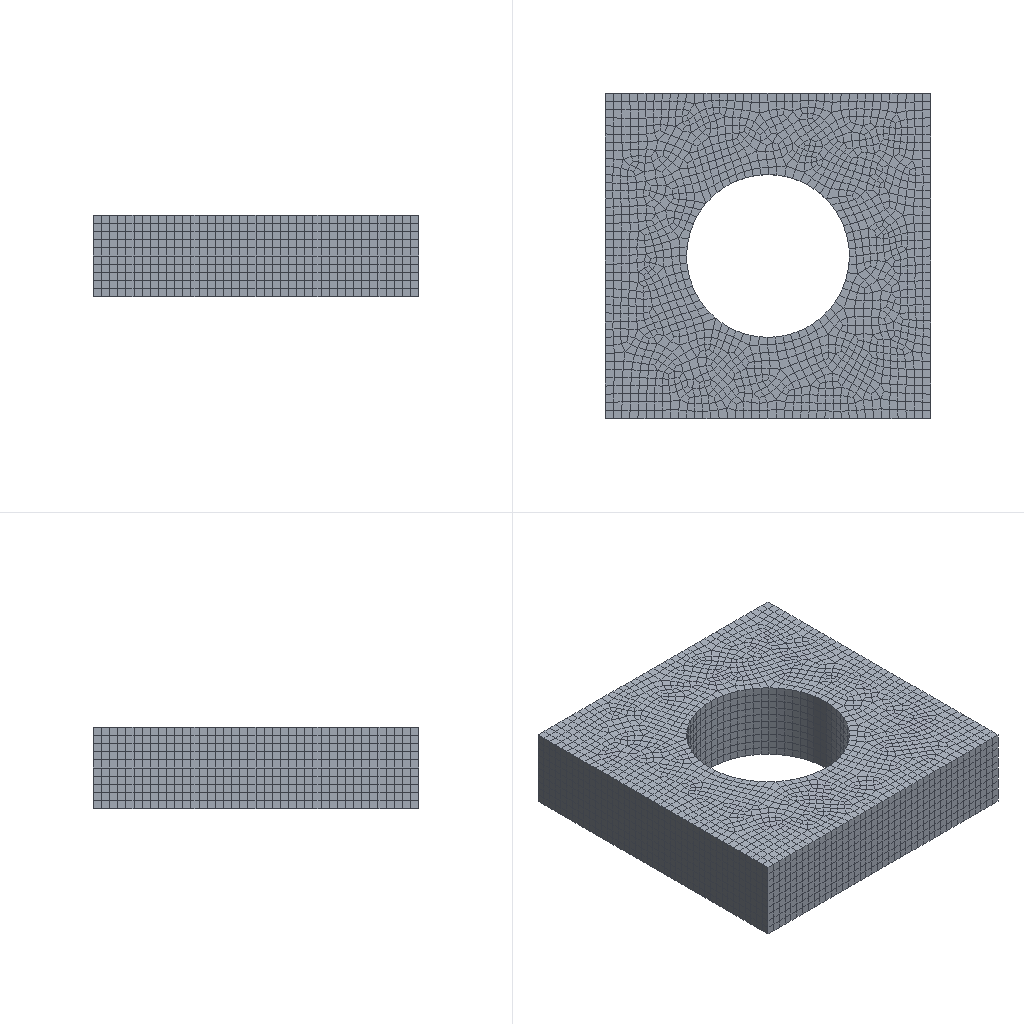Simulation study | abaqus
Set-up summary:
category,name,step,type,value,unit,region
solver,abaqus
solver,version,,,Abaqus/Explicit 2020
units,not stated in the deck,,not stated
analysis,deck,,dynamic temperature-displacement,dynamic temperature-displacement
load_step,Step-1,Step-1,dynamic temperature-displacement
load_step,requested,,,1
mesh,nodes,,,17787
mesh,elements,,,15050
element_type,C3D8RT,,solid,15050
load,load commands in deck,,count,2
bc,support commands in deck,,count,1
material,STEEL304-1,,in results
material,TOOL,,in results
check,setup vs results,,match,"per instance, exact: element labels, types and connectivity; labels of the nodes the elements use; coordinates not compared"
Abaqus input file, long lists of numbers shortened:
*Heading
** Job name: Job-2 Model name: Model-1-Copy
** Generated by: Abaqus/CAE 2020
*Preprint, echo=NO, model=NO, history=NO, contact=NO
**
** PARTS
**
*Part, name=wp
*Node
      1,  -5.688, -0.3903,           0.
      2,   -5.588, -0.2828,           0.
** (17785 more lines like these left out)
*Element, type=C3D8RT
    1,   515,   655,    33,   385,  2132,  2272,  1650,  2002
    2,   949,   243,  1108,  1056,  2566,  1860,  2725,  2673
** (15048 more lines like these left out)
*Nset, nset=_PickedSet2, internal, generate
     1,  17787,      1
*Elset, elset=_PickedSet2, internal, generate
     1,  15050,      1
** Section: wp
*Solid Section, elset=_PickedSet2, material=steel304-1
,
*End Part
**
**
** ASSEMBLY
**
*Assembly, name=Assembly
**
*Instance, name=wp-1, part=wp
          5.,           1.,           0.
*End Instance
**
*Nset, nset=Set-13, instance=wp-1, generate
     1,  17787,      1
*Elset, elset=Set-13, instance=wp-1, generate
     1,  15050,      1
*Nset, nset=Set-14, instance=wp-1, generate
     1,  17787,      1
*Elset, elset=Set-14, instance=wp-1, generate
     1,  15050,      1
*Nset, nset=Set-15, instance=wp-1, generate
     1,  17787,      1
*Elset, elset=Set-15, instance=wp-1, generate
     1,  15050,      1
*Nset, nset=s_Set-9, instance=wp-1, generate
     1,  17787,      1
*Elset, elset=s_Set-9, instance=wp-1, generate
     1,  15050,      1
*Nset, nset=s_Set-13, instance=wp-1, generate
     1,  17787,      1
*Elset, elset=s_Set-13, instance=wp-1, generate
     1,  15050,      1
*Nset, nset=_PickedSet14, internal, instance=wp-1
    22,    23,    24,    25,    26,    27,    28,    29,    30,    31,    32,    33,    34,    35,    36,    37
    38,    39,    40,    41,    42,    43,    44,    45,    46,    47,    48,    49,    50,    51,    52,    53
** (108 more lines like these left out)
*Elset, elset=_PickedSet14, internal, instance=wp-1
     1,    12,    14,    32,    36,    37,    39,    61,    63,    64,    65,    83,    85,   136,   144,   150
   151,   152,   153,   159,   165,   171,   176,   180,   187,   193,   194,   198,   206,   210,   211,   221
** (96 more lines like these left out)
*Nset, nset=_PickedSet17, internal, instance=wp-1, generate
     1,  17787,      1
*Elset, elset=_PickedSet17, internal, instance=wp-1, generate
     1,  15050,      1
*Elset, elset=_Surf-5_S5, internal, instance=wp-1
     1,    12,    32,    37,    83,    85,   144,   150,   151,   152,   165,   171,   176,   180,   187,   198
   221,   222,   223,   225,   290,   292,   300,   302,   312,   393,   563,   574,   596,   611,   615,   663
** (33 more lines like these left out)
*Elset, elset=_Surf-5_S3, internal, instance=wp-1
    14,    36,    39,   136,   153,   159,   193,   194,   230,   288,   289,   301,   471,   550,   552,   553
   554,   556,   557,   558,   559,   560,   561,   562,   565,   566,   569,   570,   572,   573,   575,   593
** (31 more lines like these left out)
*Elset, elset=_Surf-5_S6, internal, instance=wp-1
   206,   211,   229,   230,   231,   252,   470,   577,   578,   579,   580,   581,   582,   583,   585,   586
   587,   588,   589,   590,   591,   592,   594,   595,   596,   614,   615,  1711,  1716,  1734,  1735,  1736
** (15 more lines like these left out)
*Elset, elset=_Surf-5_S4, internal, instance=wp-1
    61,    63,    64,    65,   210,   232,   241,   246,   250,   253,   270,   282,   299,   305,   309,   563
   665,   668,   686,   690,   710,   726,   737,   739,   753,   757,  1566,  1568,  1569,  1570,  1715,  1737
** (15 more lines like these left out)
*Surface, type=ELEMENT, name=Surf-5
_Surf-5_S5, S5
_Surf-5_S3, S3
_Surf-5_S6, S6
_Surf-5_S4, S4
*Elset, elset=_Surf-6_S5, internal, instance=wp-1
     1,    12,    32,    37,    83,    85,   144,   150,   151,   152,   165,   171,   176,   180,   187,   198
   221,   222,   223,   225,   290,   292,   300,   302,   312,   393,   563,   574,   596,   611,   615,   663
** (33 more lines like these left out)
*Elset, elset=_Surf-6_S3, internal, instance=wp-1
    14,    36,    39,   136,   153,   159,   193,   194,   230,   288,   289,   301,   471,   550,   552,   553
   554,   556,   557,   558,   559,   560,   561,   562,   565,   566,   569,   570,   572,   573,   575,   593
** (31 more lines like these left out)
*Elset, elset=_Surf-6_S6, internal, instance=wp-1
   206,   211,   229,   230,   231,   252,   470,   577,   578,   579,   580,   581,   582,   583,   585,   586
   587,   588,   589,   590,   591,   592,   594,   595,   596,   614,   615,  1711,  1716,  1734,  1735,  1736
** (15 more lines like these left out)
*Elset, elset=_Surf-6_S4, internal, instance=wp-1
    61,    63,    64,    65,   210,   232,   241,   246,   250,   253,   270,   282,   299,   305,   309,   563
   665,   668,   686,   690,   710,   726,   737,   739,   753,   757,  1566,  1568,  1569,  1570,  1715,  1737
** (15 more lines like these left out)
*Surface, type=ELEMENT, name=Surf-6
_Surf-6_S5, S5
_Surf-6_S3, S3
_Surf-6_S6, S6
_Surf-6_S4, S4
*Elset, elset=_Surf-9_S3, internal, instance=wp-1
     4,     5,     6,    14,    36,    39,    45,    49,    51,    92,    95,   100,   108,   111,   133,   134
   136,   153,   159,   164,   185,   193,   194,   205,   230,   288,   289,   301,   389,   412,   421,   471
** (50 more lines like these left out)
*Elset, elset=_Surf-9_S5, internal, instance=wp-1
     1,    12,    24,    25,    32,    37,    50,    52,    83,    85,    93,   105,   107,   127,   128,   129
   135,   144,   150,   151,   152,   165,   171,   176,   180,   187,   198,   221,   222,   223,   225,   290
** (45 more lines like these left out)
*Elset, elset=_Surf-9_S6, internal, instance=wp-1
    53,    54,    55,   104,   109,   206,   211,   229,   230,   231,   252,   344,   353,   470,   527,   536
   547,   577,   578,   579,   580,   581,   582,   583,   585,   586,   587,   588,   589,   590,   591,   592
** (22 more lines like these left out)
*Elset, elset=_Surf-9_S4, internal, instance=wp-1
    61,    63,    64,    65,   124,   125,   130,   210,   232,   241,   246,   250,   253,   270,   282,   299
   305,   309,   343,   530,   563,   665,   668,   686,   690,   710,   726,   737,   739,   753,   757,  1566
** (18 more lines like these left out)
*Elset, elset=_Surf-9_S2, internal, instance=wp-1, generate
 13546,  15050,      1
*Elset, elset=_Surf-9_S1, internal, instance=wp-1, generate
    1,  1505,     1
*Surface, type=ELEMENT, name=Surf-9
_Surf-9_S3, S3
_Surf-9_S5, S5
_Surf-9_S6, S6
_Surf-9_S4, S4
_Surf-9_S2, S2
_Surf-9_S1, S1
*Elset, elset=_Surf-10_S3, internal, instance=wp-1
     4,     5,     6,    14,    36,    39,    45,    49,    51,    92,    95,   100,   108,   111,   133,   134
   136,   153,   159,   164,   185,   193,   194,   205,   230,   288,   289,   301,   389,   412,   421,   471
** (50 more lines like these left out)
*Elset, elset=_Surf-10_S5, internal, instance=wp-1
     1,    12,    24,    25,    32,    37,    50,    52,    83,    85,    93,   105,   107,   127,   128,   129
   135,   144,   150,   151,   152,   165,   171,   176,   180,   187,   198,   221,   222,   223,   225,   290
** (45 more lines like these left out)
*Elset, elset=_Surf-10_S6, internal, instance=wp-1
    53,    54,    55,   104,   109,   206,   211,   229,   230,   231,   252,   344,   353,   470,   527,   536
   547,   577,   578,   579,   580,   581,   582,   583,   585,   586,   587,   588,   589,   590,   591,   592
** (22 more lines like these left out)
*Elset, elset=_Surf-10_S4, internal, instance=wp-1
    61,    63,    64,    65,   124,   125,   130,   210,   232,   241,   246,   250,   253,   270,   282,   299
   305,   309,   343,   530,   563,   665,   668,   686,   690,   710,   726,   737,   739,   753,   757,  1566
** (18 more lines like these left out)
*Elset, elset=_Surf-10_S2, internal, instance=wp-1, generate
 13546,  15050,      1
*Elset, elset=_Surf-10_S1, internal, instance=wp-1, generate
    1,  1505,     1
*Surface, type=ELEMENT, name=Surf-10
_Surf-10_S3, S3
_Surf-10_S5, S5
_Surf-10_S6, S6
_Surf-10_S4, S4
_Surf-10_S2, S2
_Surf-10_S1, S1
*Elset, elset=__PickedSurf16_S5, internal, instance=wp-1
    37,   144,   180,   187,   198,   221,   222,   223,   225,   290,   292,   300,   302,   312,   574,   596
   611,   717,   721,   724,   729,   730,   732,   734,   738,   742,   743,   746,   747,   748,   749,   750
** (20 more lines like these left out)
*Elset, elset=__PickedSurf16_S3, internal, instance=wp-1
    39,   193,   194,   230,   288,   289,   301,   565,   566,   569,   570,   572,   573,   575,   599,   600
   601,   604,   605,   606,   607,   609,   610,   612,   760,   762,   764,   767,   769,   771,   773,   776
** (18 more lines like these left out)
*Elset, elset=__PickedSurf16_S6, internal, instance=wp-1
   229,   470,   577,   578,   614,   615,  1734,  1975,  2082,  2083,  2119,  2120,  3239,  3480,  3587,  3588
  3624,  3625,  4744,  4985,  5092,  5093,  5129,  5130,  6249,  6490,  6597,  6598,  6634,  6635,  7754,  7995
** (2 more lines like these left out)
*Elset, elset=__PickedSurf16_S4, internal, instance=wp-1
   305,   309,   563,   726,   737,   739,   753,   757,  1810,  1814,  2068,  2231,  2242,  2244,  2258,  2262
  3315,  3319,  3573,  3736,  3747,  3749,  3763,  3767,  4820,  4824,  5078,  5241,  5252,  5254,  5268,  5272
** (3 more lines like these left out)
*Surface, type=ELEMENT, name=_PickedSurf16, internal
__PickedSurf16_S5, S5
__PickedSurf16_S3, S3
__PickedSurf16_S6, S6
__PickedSurf16_S4, S4
*End Assembly
*Amplitude, name=Amp-1
             0.,              1.,             5.5,              1.
**
** MATERIALS
**
*Material, name=steel304-1
*Conductivity
16.,
*Density
 7.93e-09,
*Elastic
198000., 0.3
*Expansion
 1.73e-05,
*Inelastic Heat Fraction
         0.9,
*Specific Heat
 5e+08,
*Material, name=tool
*Conductivity
75.,
*Density
 1.45e-08,
*Elastic
640000., 0.22
*Plastic
608.,0.
*Specific Heat
 2.2e+08,
**
** INTERACTION PROPERTIES
**
*Surface Interaction, name=IntProp-1
*Friction
 0.3,
*Surface Behavior, pressure-overclosure=HARD
*Gap Heat Generation
1., 0.5
**
** PHYSICAL CONSTANTS
**
*Physical Constants, absolute zero=-273., stefan boltzmann=5.67e-08
**
** BOUNDARY CONDITIONS
**
** Name: [REDACTED] : Symmetric / antisymmetric / fully fixed
*Boundary
_PickedSet14, ENCASTRE
**
** PREDEFINED FIELDS
**
** Name: Predefined Field-1   Type: Temperature
*Initial Conditions, type=TEMPERATURE, file=D:\_____________\_____\_____._______________________
** Name: Predefined Field-2   Type: Stress
*Initial Conditions, type=STRESS, file=D:/_____________/_____/_____._______________________
** ----------------------------------------------------------------
**
** STEP: Step-1
**
*Step, name=Step-1, nlgeom=YES
*Dynamic Temperature-displacement, Explicit
, 0.1
*Bulk Viscosity
0.06, 1.2
** Mass Scaling: Semi-Automatic
**               Whole Model
*Fixed Mass Scaling, factor=5000.
*Adaptive Mesh Controls, name=Ada-1, geometric enhancement=YES
1., 0., 0.
*Adaptive Mesh, elset=_PickedSet17, controls=Ada-1, frequency=30, mesh sweeps=10, op=NEW
**
** INTERACTIONS
**
** Interaction: Int-2
*Sradiate
Surf-9, R, 20., 0.8
** Interaction: Int-3
*Sfilm
Surf-10, F, 20., 0.05
**
** OUTPUT REQUESTS
**
*Restart, write, number interval=1, time marks=NO
**
** FIELD OUTPUT: F-Output-1
**
*Output, field, number interval=100
*Node Output
NT, RF, RM, RT, U, V
*Element Output, directions=YES
E, HFL, LE, MISES, PE, PEEQ, S, STATUS, TEMP
*Contact Output
CSTRESS,
**
** HISTORY OUTPUT: H-Output-1
**
*Output, history, variable=PRESELECT
*End Step
Results summary:
result,step,Step-1,completed,increments=424510 time=0.1/0.1
result,analysis,,,"dynamic temperature-displacement, explict"
result,last_loadstep,,,1
result,primary field,,,"U, NT11"
result,reaction total,,FX,0.001893,model units
result,reaction total,,FY,-0.002379,model units
result,reaction total,,FZ,0.03378,model units